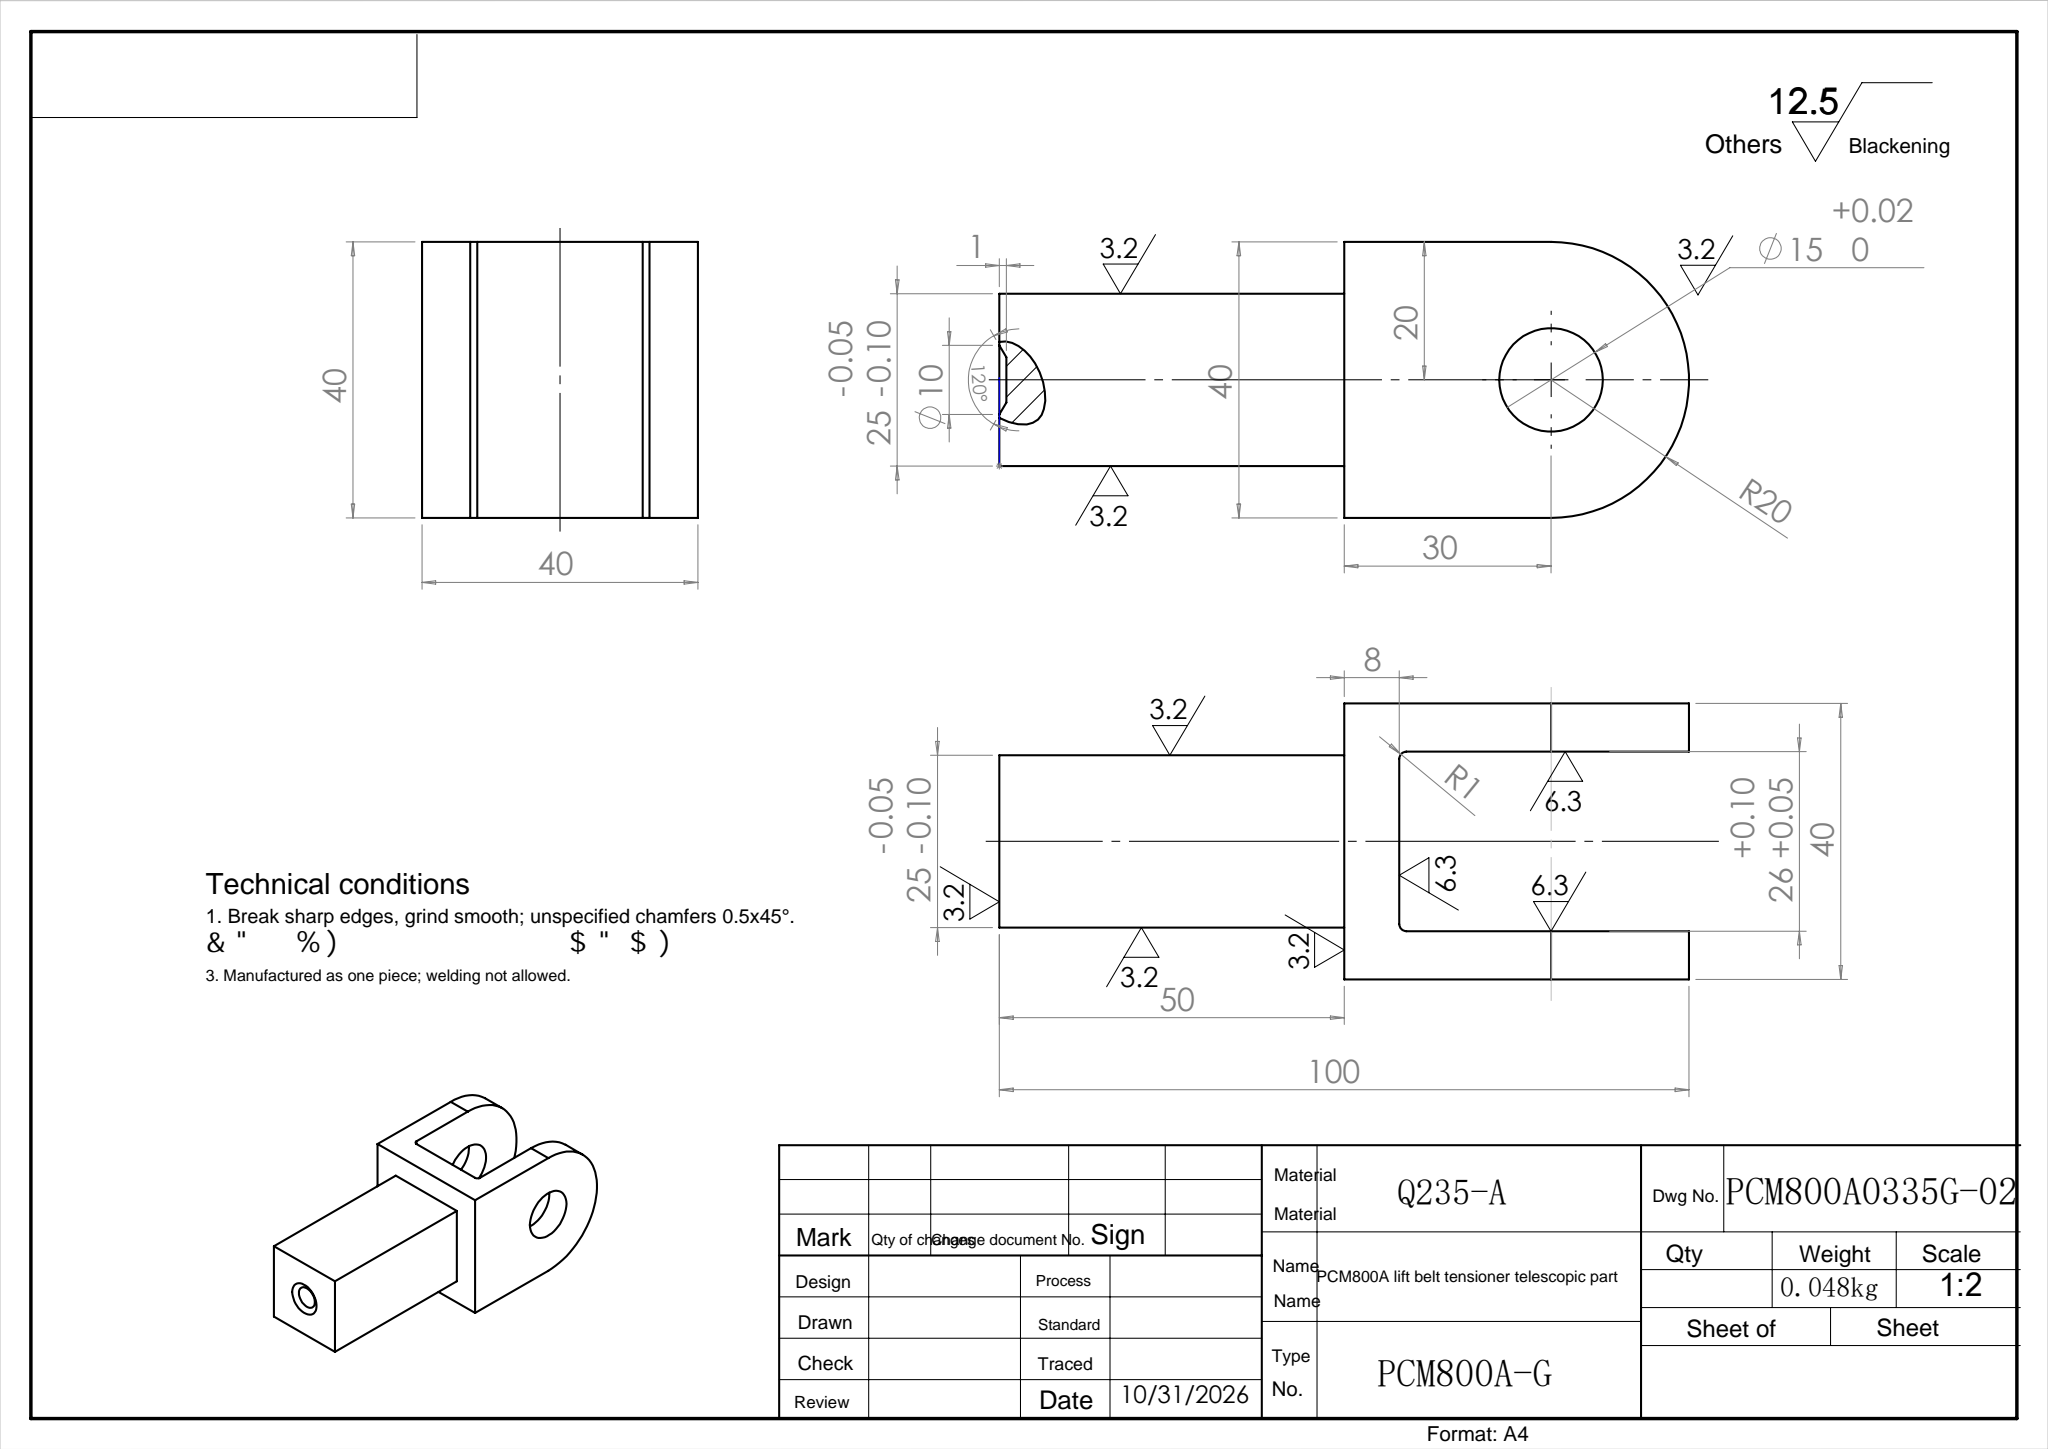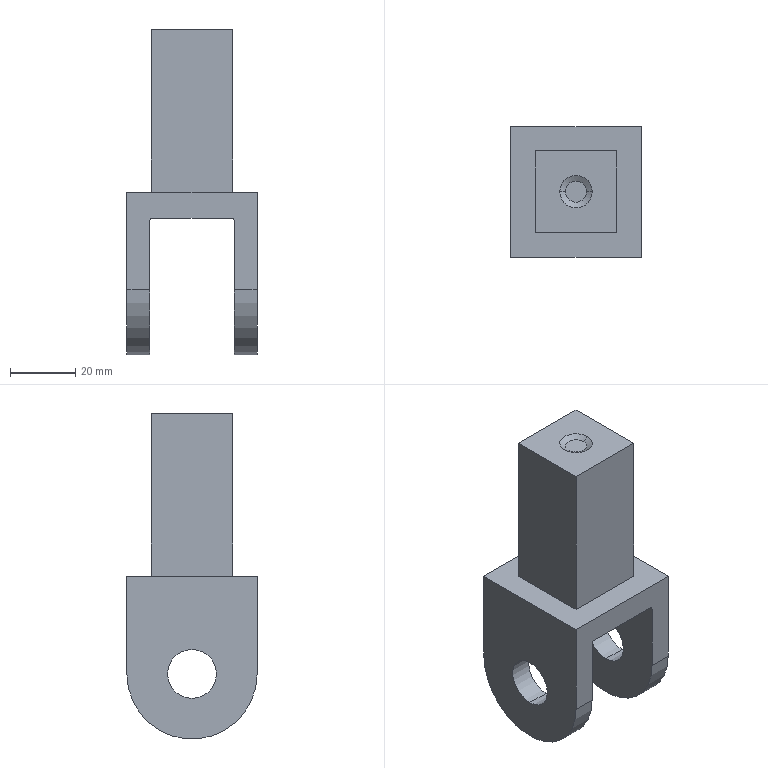Part | SolidWorks | features Fillet 1, MirrorStock 1 | 1 solid | 24 faces | box 40 x 40 x 100 mm | volume 62655 mm3 | plane 14 | cylinder 8 | cone 2 | commonest cylinder face diameters 15 x4 2 x2 40 x2
STEP:
#1=CARTESIAN_POINT('',(9.232,12.5,-1.));
#2=VERTEX_POINT('',#1);
#3=CARTESIAN_POINT('',(15.768,12.5,-1.));
#4=VERTEX_POINT('',#3);
#5=CARTESIAN_POINT('',(12.5,12.5,-1.));
#6=DIRECTION('',(0.,0.,-1.));
#7=DIRECTION('',(-1.,0.,0.));
#8=AXIS2_PLACEMENT_3D('',#5,#6,#7);
#9=CIRCLE('',#8,3.268);
#10=EDGE_CURVE('',#2,#4,#9,.T.);
#11=ORIENTED_EDGE('',*,*,#10,.T.);
#12=CARTESIAN_POINT('',(17.5,12.5,0.));
#13=VERTEX_POINT('',#12);
#14=CARTESIAN_POINT('',(17.5,12.5,0.));
#15=DIRECTION('',(0.866,0.,0.5));
#16=VECTOR('',#15,1000.);
#17=LINE('',#14,#16);
#18=EDGE_CURVE('',#4,#13,#17,.T.);
#19=ORIENTED_EDGE('',*,*,#18,.T.);
#20=CARTESIAN_POINT('',(7.5,12.5,0.));
#21=VERTEX_POINT('',#20);
#22=CARTESIAN_POINT('',(12.5,12.5,0.));
#23=DIRECTION('',(0.,0.,-1.));
#24=DIRECTION('',(-1.,0.,0.));
#25=AXIS2_PLACEMENT_3D('',#22,#23,#24);
#26=CIRCLE('',#25,5.);
#27=EDGE_CURVE('',#21,#13,#26,.T.);
#28=ORIENTED_EDGE('',*,*,#27,.F.);
#29=CARTESIAN_POINT('',(7.5,12.5,0.));
#30=DIRECTION('',(-0.866,0.,0.5));
#31=VECTOR('',#30,1000.);
#32=LINE('',#29,#31);
#33=EDGE_CURVE('',#2,#21,#32,.T.);
#34=ORIENTED_EDGE('',*,*,#33,.F.);
#35=EDGE_LOOP('',(#11,#19,#28,#34));
#36=FACE_OUTER_BOUND('',#35,.T.);
#37=CARTESIAN_POINT('',(12.5,12.5,0.));
#38=DIRECTION('',(0.,0.,1.));
#39=DIRECTION('',(-1.,0.,0.));
#40=AXIS2_PLACEMENT_3D('',#37,#38,#39);
#41=CONICAL_SURFACE('',#40,5.,1.047);
#42=ADVANCED_FACE('',(#36),#41,.F.);
#43=CARTESIAN_POINT('',(25.5,12.5,-72.5));
#44=VERTEX_POINT('',#43);
#45=CARTESIAN_POINT('',(25.5,12.5,-87.5));
#46=VERTEX_POINT('',#45);
#47=CARTESIAN_POINT('',(25.5,12.5,-80.));
#48=DIRECTION('',(-1.,0.,0.));
#49=DIRECTION('',(0.,1.,0.));
#50=AXIS2_PLACEMENT_3D('',#47,#48,#49);
#51=CIRCLE('',#50,7.5);
#52=EDGE_CURVE('',#44,#46,#51,.T.);
#53=ORIENTED_EDGE('',*,*,#52,.T.);
#54=CARTESIAN_POINT('',(32.5,12.5,-87.5));
#55=VERTEX_POINT('',#54);
#56=CARTESIAN_POINT('',(-7.5,12.5,-87.5));
#57=DIRECTION('',(1.,0.,0.));
#58=VECTOR('',#57,1000.);
#59=LINE('',#56,#58);
#60=EDGE_CURVE('',#46,#55,#59,.T.);
#61=ORIENTED_EDGE('',*,*,#60,.T.);
#62=CARTESIAN_POINT('',(32.5,12.5,-72.5));
#63=VERTEX_POINT('',#62);
#64=CARTESIAN_POINT('',(32.5,12.5,-80.));
#65=DIRECTION('',(-1.,0.,0.));
#66=DIRECTION('',(0.,0.,1.));
#67=AXIS2_PLACEMENT_3D('',#64,#65,#66);
#68=CIRCLE('',#67,7.5);
#69=EDGE_CURVE('',#63,#55,#68,.T.);
#70=ORIENTED_EDGE('',*,*,#69,.F.);
#71=CARTESIAN_POINT('',(-7.5,12.5,-72.5));
#72=DIRECTION('',(1.,0.,0.));
#73=VECTOR('',#72,1000.);
#74=LINE('',#71,#73);
#75=EDGE_CURVE('',#44,#63,#74,.T.);
#76=ORIENTED_EDGE('',*,*,#75,.F.);
#77=EDGE_LOOP('',(#53,#61,#70,#76));
#78=FACE_OUTER_BOUND('',#77,.T.);
#79=CARTESIAN_POINT('',(-7.5,12.5,-80.));
#80=DIRECTION('',(1.,0.,0.));
#81=DIRECTION('',(0.,0.,1.));
#82=AXIS2_PLACEMENT_3D('',#79,#80,#81);
#83=CYLINDRICAL_SURFACE('',#82,7.5);
#84=ADVANCED_FACE('',(#78),#83,.F.);
#85=CARTESIAN_POINT('',(-7.5,12.5,-72.5));
#86=VERTEX_POINT('',#85);
#87=CARTESIAN_POINT('',(-7.5,12.5,-87.5));
#88=VERTEX_POINT('',#87);
#89=CARTESIAN_POINT('',(-7.5,12.5,-80.));
#90=DIRECTION('',(-1.,0.,0.));
#91=DIRECTION('',(0.,0.,1.));
#92=AXIS2_PLACEMENT_3D('',#89,#90,#91);
#93=CIRCLE('',#92,7.5);
#94=EDGE_CURVE('',#86,#88,#93,.T.);
#95=ORIENTED_EDGE('',*,*,#94,.T.);
#96=CARTESIAN_POINT('',(-0.5,12.5,-87.5));
#97=VERTEX_POINT('',#96);
#98=CARTESIAN_POINT('',(-7.5,12.5,-87.5));
#99=DIRECTION('',(1.,0.,0.));
#100=VECTOR('',#99,1000.);
#101=LINE('',#98,#100);
#102=EDGE_CURVE('',#88,#97,#101,.T.);
#103=ORIENTED_EDGE('',*,*,#102,.T.);
#104=CARTESIAN_POINT('',(-0.5,12.5,-72.5));
#105=VERTEX_POINT('',#104);
#106=CARTESIAN_POINT('',(-0.5,12.5,-80.));
#107=DIRECTION('',(1.,0.,0.));
#108=DIRECTION('',(0.,-1.,0.));
#109=AXIS2_PLACEMENT_3D('',#106,#107,#108);
#110=CIRCLE('',#109,7.5);
#111=EDGE_CURVE('',#97,#105,#110,.T.);
#112=ORIENTED_EDGE('',*,*,#111,.T.);
#113=CARTESIAN_POINT('',(-7.5,12.5,-72.5));
#114=DIRECTION('',(1.,0.,0.));
#115=VECTOR('',#114,1000.);
#116=LINE('',#113,#115);
#117=EDGE_CURVE('',#86,#105,#116,.T.);
#118=ORIENTED_EDGE('',*,*,#117,.F.);
#119=EDGE_LOOP('',(#95,#103,#112,#118));
#120=FACE_OUTER_BOUND('',#119,.T.);
#121=CARTESIAN_POINT('',(-7.5,12.5,-80.));
#122=DIRECTION('',(1.,0.,0.));
#123=DIRECTION('',(0.,0.,1.));
#124=AXIS2_PLACEMENT_3D('',#121,#122,#123);
#125=CYLINDRICAL_SURFACE('',#124,7.5);
#126=ADVANCED_FACE('',(#120),#125,.F.);
#127=CARTESIAN_POINT('',(25.5,-7.5,-80.));
#128=VERTEX_POINT('',#127);
#129=CARTESIAN_POINT('',(25.5,32.5,-80.));
#130=VERTEX_POINT('',#129);
#131=CARTESIAN_POINT('',(25.5,12.5,-80.));
#132=DIRECTION('',(1.,0.,0.));
#133=DIRECTION('',(0.,1.,0.));
#134=AXIS2_PLACEMENT_3D('',#131,#132,#133);
#135=CIRCLE('',#134,20.);
#136=EDGE_CURVE('',#128,#130,#135,.T.);
#137=ORIENTED_EDGE('',*,*,#136,.T.);
#138=CARTESIAN_POINT('',(32.5,32.5,-80.));
#139=VERTEX_POINT('',#138);
#140=CARTESIAN_POINT('',(-17.5,32.5,-80.));
#141=DIRECTION('',(1.,0.,0.));
#142=VECTOR('',#141,1000.);
#143=LINE('',#140,#142);
#144=EDGE_CURVE('',#130,#139,#143,.T.);
#145=ORIENTED_EDGE('',*,*,#144,.T.);
#146=CARTESIAN_POINT('',(32.5,-7.5,-80.));
#147=VERTEX_POINT('',#146);
#148=CARTESIAN_POINT('',(32.5,12.5,-80.));
#149=DIRECTION('',(-1.,0.,0.));
#150=DIRECTION('',(0.,0.,1.));
#151=AXIS2_PLACEMENT_3D('',#148,#149,#150);
#152=CIRCLE('',#151,20.);
#153=EDGE_CURVE('',#139,#147,#152,.T.);
#154=ORIENTED_EDGE('',*,*,#153,.T.);
#155=CARTESIAN_POINT('',(-17.5,-7.5,-80.));
#156=DIRECTION('',(1.,0.,0.));
#157=VECTOR('',#156,1000.);
#158=LINE('',#155,#157);
#159=EDGE_CURVE('',#128,#147,#158,.T.);
#160=ORIENTED_EDGE('',*,*,#159,.F.);
#161=EDGE_LOOP('',(#137,#145,#154,#160));
#162=FACE_OUTER_BOUND('',#161,.T.);
#163=CARTESIAN_POINT('',(-17.5,12.5,-80.));
#164=DIRECTION('',(1.,0.,0.));
#165=DIRECTION('',(0.,0.,1.));
#166=AXIS2_PLACEMENT_3D('',#163,#164,#165);
#167=CYLINDRICAL_SURFACE('',#166,20.);
#168=ADVANCED_FACE('',(#162),#167,.T.);
#169=ORIENTED_EDGE('',*,*,#94,.F.);
#170=CARTESIAN_POINT('',(-7.5,12.5,-80.));
#171=DIRECTION('',(-1.,0.,0.));
#172=DIRECTION('',(0.,0.,1.));
#173=AXIS2_PLACEMENT_3D('',#170,#171,#172);
#174=CIRCLE('',#173,7.5);
#175=EDGE_CURVE('',#88,#86,#174,.T.);
#176=ORIENTED_EDGE('',*,*,#175,.F.);
#177=EDGE_LOOP('',(#169,#176));
#178=FACE_BOUND('',#177,.T.);
#179=CARTESIAN_POINT('',(-7.5,32.5,-80.));
#180=VERTEX_POINT('',#179);
#181=CARTESIAN_POINT('',(-7.5,-7.5,-80.));
#182=VERTEX_POINT('',#181);
#183=CARTESIAN_POINT('',(-7.5,12.5,-80.));
#184=DIRECTION('',(-1.,0.,0.));
#185=DIRECTION('',(0.,1.,0.));
#186=AXIS2_PLACEMENT_3D('',#183,#184,#185);
#187=CIRCLE('',#186,20.);
#188=EDGE_CURVE('',#180,#182,#187,.T.);
#189=ORIENTED_EDGE('',*,*,#188,.T.);
#190=CARTESIAN_POINT('',(-7.5,-7.5,-50.));
#191=VERTEX_POINT('',#190);
#192=CARTESIAN_POINT('',(-7.5,-7.5,-100.));
#193=DIRECTION('',(0.,0.,1.));
#194=VECTOR('',#193,1000.);
#195=LINE('',#192,#194);
#196=EDGE_CURVE('',#182,#191,#195,.T.);
#197=ORIENTED_EDGE('',*,*,#196,.T.);
#198=CARTESIAN_POINT('',(-7.5,32.5,-50.));
#199=VERTEX_POINT('',#198);
#200=CARTESIAN_POINT('',(-7.5,32.5,-50.));
#201=DIRECTION('',(0.,-1.,0.));
#202=VECTOR('',#201,1000.);
#203=LINE('',#200,#202);
#204=EDGE_CURVE('',#199,#191,#203,.T.);
#205=ORIENTED_EDGE('',*,*,#204,.F.);
#206=CARTESIAN_POINT('',(-7.5,32.5,-100.));
#207=DIRECTION('',(0.,0.,1.));
#208=VECTOR('',#207,1000.);
#209=LINE('',#206,#208);
#210=EDGE_CURVE('',#180,#199,#209,.T.);
#211=ORIENTED_EDGE('',*,*,#210,.F.);
#212=EDGE_LOOP('',(#189,#197,#205,#211));
#213=FACE_OUTER_BOUND('',#212,.T.);
#214=CARTESIAN_POINT('',(-7.5,32.5,-100.));
#215=DIRECTION('',(1.,0.,0.));
#216=DIRECTION('',(0.,1.,0.));
#217=AXIS2_PLACEMENT_3D('',#214,#215,#216);
#218=PLANE('',#217);
#219=ADVANCED_FACE('',(#178,#213),#218,.F.);
#220=ORIENTED_EDGE('',*,*,#69,.T.);
#221=CARTESIAN_POINT('',(32.5,12.5,-80.));
#222=DIRECTION('',(-1.,0.,0.));
#223=DIRECTION('',(0.,0.,1.));
#224=AXIS2_PLACEMENT_3D('',#221,#222,#223);
#225=CIRCLE('',#224,7.5);
#226=EDGE_CURVE('',#55,#63,#225,.T.);
#227=ORIENTED_EDGE('',*,*,#226,.T.);
#228=EDGE_LOOP('',(#220,#227));
#229=FACE_BOUND('',#228,.T.);
#230=CARTESIAN_POINT('',(32.5,32.5,-50.));
#231=VERTEX_POINT('',#230);
#232=CARTESIAN_POINT('',(32.5,32.5,-100.));
#233=DIRECTION('',(0.,0.,1.));
#234=VECTOR('',#233,1000.);
#235=LINE('',#232,#234);
#236=EDGE_CURVE('',#139,#231,#235,.T.);
#237=ORIENTED_EDGE('',*,*,#236,.T.);
#238=CARTESIAN_POINT('',(32.5,-7.5,-50.));
#239=VERTEX_POINT('',#238);
#240=CARTESIAN_POINT('',(32.5,32.5,-50.));
#241=DIRECTION('',(0.,1.,0.));
#242=VECTOR('',#241,1000.);
#243=LINE('',#240,#242);
#244=EDGE_CURVE('',#239,#231,#243,.T.);
#245=ORIENTED_EDGE('',*,*,#244,.F.);
#246=CARTESIAN_POINT('',(32.5,-7.5,-100.));
#247=DIRECTION('',(0.,0.,1.));
#248=VECTOR('',#247,1000.);
#249=LINE('',#246,#248);
#250=EDGE_CURVE('',#147,#239,#249,.T.);
#251=ORIENTED_EDGE('',*,*,#250,.F.);
#252=ORIENTED_EDGE('',*,*,#153,.F.);
#253=EDGE_LOOP('',(#237,#245,#251,#252));
#254=FACE_OUTER_BOUND('',#253,.T.);
#255=CARTESIAN_POINT('',(32.5,32.5,-100.));
#256=DIRECTION('',(-1.,0.,0.));
#257=DIRECTION('',(0.,0.,-1.));
#258=AXIS2_PLACEMENT_3D('',#255,#256,#257);
#259=PLANE('',#258);
#260=ADVANCED_FACE('',(#229,#254),#259,.F.);
#261=ORIENTED_EDGE('',*,*,#159,.T.);
#262=ORIENTED_EDGE('',*,*,#250,.T.);
#263=CARTESIAN_POINT('',(-7.5,-7.5,-50.));
#264=DIRECTION('',(1.,0.,0.));
#265=VECTOR('',#264,1000.);
#266=LINE('',#263,#265);
#267=EDGE_CURVE('',#191,#239,#266,.T.);
#268=ORIENTED_EDGE('',*,*,#267,.F.);
#269=ORIENTED_EDGE('',*,*,#196,.F.);
#270=CARTESIAN_POINT('',(-0.5,-7.5,-80.));
#271=VERTEX_POINT('',#270);
#272=CARTESIAN_POINT('',(-17.5,-7.5,-80.));
#273=DIRECTION('',(1.,0.,0.));
#274=VECTOR('',#273,1000.);
#275=LINE('',#272,#274);
#276=EDGE_CURVE('',#182,#271,#275,.T.);
#277=ORIENTED_EDGE('',*,*,#276,.T.);
#278=CARTESIAN_POINT('',(-0.5,-7.5,-59.));
#279=VERTEX_POINT('',#278);
#280=CARTESIAN_POINT('',(-0.5,-7.5,-58.));
#281=DIRECTION('',(0.,0.,-1.));
#282=VECTOR('',#281,1000.);
#283=LINE('',#280,#282);
#284=EDGE_CURVE('',#279,#271,#283,.T.);
#285=ORIENTED_EDGE('',*,*,#284,.F.);
#286=CARTESIAN_POINT('',(0.5,-7.5,-58.));
#287=VERTEX_POINT('',#286);
#288=CARTESIAN_POINT('',(0.5,-7.5,-59.));
#289=DIRECTION('',(0.,1.,0.));
#290=DIRECTION('',(0.,0.,1.));
#291=AXIS2_PLACEMENT_3D('',#288,#289,#290);
#292=CIRCLE('',#291,1.);
#293=EDGE_CURVE('',#279,#287,#292,.T.);
#294=ORIENTED_EDGE('',*,*,#293,.T.);
#295=CARTESIAN_POINT('',(24.5,-7.5,-58.));
#296=VERTEX_POINT('',#295);
#297=CARTESIAN_POINT('',(25.5,-7.5,-58.));
#298=DIRECTION('',(-1.,0.,0.));
#299=VECTOR('',#298,1000.);
#300=LINE('',#297,#299);
#301=EDGE_CURVE('',#296,#287,#300,.T.);
#302=ORIENTED_EDGE('',*,*,#301,.F.);
#303=CARTESIAN_POINT('',(25.5,-7.5,-59.));
#304=VERTEX_POINT('',#303);
#305=CARTESIAN_POINT('',(24.5,-7.5,-59.));
#306=DIRECTION('',(0.,1.,0.));
#307=DIRECTION('',(0.,0.,1.));
#308=AXIS2_PLACEMENT_3D('',#305,#306,#307);
#309=CIRCLE('',#308,1.);
#310=EDGE_CURVE('',#296,#304,#309,.T.);
#311=ORIENTED_EDGE('',*,*,#310,.T.);
#312=CARTESIAN_POINT('',(25.5,-7.5,-58.));
#313=DIRECTION('',(0.,0.,1.));
#314=VECTOR('',#313,1000.);
#315=LINE('',#312,#314);
#316=EDGE_CURVE('',#128,#304,#315,.T.);
#317=ORIENTED_EDGE('',*,*,#316,.F.);
#318=EDGE_LOOP('',(#261,#262,#268,#269,#277,#285,#294,#302,#311,#317));
#319=FACE_OUTER_BOUND('',#318,.T.);
#320=CARTESIAN_POINT('',(-7.5,-7.5,-100.));
#321=DIRECTION('',(0.,1.,0.));
#322=DIRECTION('',(0.,0.,-1.));
#323=AXIS2_PLACEMENT_3D('',#320,#321,#322);
#324=PLANE('',#323);
#325=ADVANCED_FACE('',(#319),#324,.F.);
#326=CARTESIAN_POINT('',(0.,25.,0.));
#327=VERTEX_POINT('',#326);
#328=CARTESIAN_POINT('',(0.,0.,0.));
#329=VERTEX_POINT('',#328);
#330=CARTESIAN_POINT('',(0.,0.,0.));
#331=DIRECTION('',(0.,-1.,0.));
#332=VECTOR('',#331,1000.);
#333=LINE('',#330,#332);
#334=EDGE_CURVE('',#327,#329,#333,.T.);
#335=ORIENTED_EDGE('',*,*,#334,.F.);
#336=CARTESIAN_POINT('',(0.,25.,-50.));
#337=VERTEX_POINT('',#336);
#338=CARTESIAN_POINT('',(0.,25.,-50.));
#339=DIRECTION('',(0.,0.,1.));
#340=VECTOR('',#339,1000.);
#341=LINE('',#338,#340);
#342=EDGE_CURVE('',#337,#327,#341,.T.);
#343=ORIENTED_EDGE('',*,*,#342,.F.);
#344=CARTESIAN_POINT('',(0.,0.,-50.));
#345=VERTEX_POINT('',#344);
#346=CARTESIAN_POINT('',(0.,0.,-50.));
#347=DIRECTION('',(0.,-1.,0.));
#348=VECTOR('',#347,1000.);
#349=LINE('',#346,#348);
#350=EDGE_CURVE('',#337,#345,#349,.T.);
#351=ORIENTED_EDGE('',*,*,#350,.T.);
#352=CARTESIAN_POINT('',(0.,0.,-50.));
#353=DIRECTION('',(0.,0.,1.));
#354=VECTOR('',#353,1000.);
#355=LINE('',#352,#354);
#356=EDGE_CURVE('',#345,#329,#355,.T.);
#357=ORIENTED_EDGE('',*,*,#356,.T.);
#358=EDGE_LOOP('',(#335,#343,#351,#357));
#359=FACE_OUTER_BOUND('',#358,.T.);
#360=CARTESIAN_POINT('',(0.,0.,-50.));
#361=DIRECTION('',(1.,0.,0.));
#362=DIRECTION('',(0.,0.,1.));
#363=AXIS2_PLACEMENT_3D('',#360,#361,#362);
#364=PLANE('',#363);
#365=ADVANCED_FACE('',(#359),#364,.F.);
#366=CARTESIAN_POINT('',(25.,0.,0.));
#367=VERTEX_POINT('',#366);
#368=CARTESIAN_POINT('',(0.,0.,0.));
#369=DIRECTION('',(1.,0.,0.));
#370=VECTOR('',#369,1000.);
#371=LINE('',#368,#370);
#372=EDGE_CURVE('',#329,#367,#371,.T.);
#373=ORIENTED_EDGE('',*,*,#372,.F.);
#374=ORIENTED_EDGE('',*,*,#356,.F.);
#375=CARTESIAN_POINT('',(25.,0.,-50.));
#376=VERTEX_POINT('',#375);
#377=CARTESIAN_POINT('',(0.,0.,-50.));
#378=DIRECTION('',(1.,0.,0.));
#379=VECTOR('',#378,1000.);
#380=LINE('',#377,#379);
#381=EDGE_CURVE('',#345,#376,#380,.T.);
#382=ORIENTED_EDGE('',*,*,#381,.T.);
#383=CARTESIAN_POINT('',(25.,0.,-50.));
#384=DIRECTION('',(0.,0.,1.));
#385=VECTOR('',#384,1000.);
#386=LINE('',#383,#385);
#387=EDGE_CURVE('',#376,#367,#386,.T.);
#388=ORIENTED_EDGE('',*,*,#387,.T.);
#389=EDGE_LOOP('',(#373,#374,#382,#388));
#390=FACE_OUTER_BOUND('',#389,.T.);
#391=CARTESIAN_POINT('',(0.,0.,-50.));
#392=DIRECTION('',(0.,1.,0.));
#393=DIRECTION('',(0.,0.,-1.));
#394=AXIS2_PLACEMENT_3D('',#391,#392,#393);
#395=PLANE('',#394);
#396=ADVANCED_FACE('',(#390),#395,.F.);
#397=CARTESIAN_POINT('',(25.,25.,0.));
#398=VERTEX_POINT('',#397);
#399=CARTESIAN_POINT('',(25.,0.,0.));
#400=DIRECTION('',(0.,1.,0.));
#401=VECTOR('',#400,1000.);
#402=LINE('',#399,#401);
#403=EDGE_CURVE('',#367,#398,#402,.T.);
#404=ORIENTED_EDGE('',*,*,#403,.F.);
#405=ORIENTED_EDGE('',*,*,#387,.F.);
#406=CARTESIAN_POINT('',(25.,25.,-50.));
#407=VERTEX_POINT('',#406);
#408=CARTESIAN_POINT('',(25.,0.,-50.));
#409=DIRECTION('',(0.,1.,0.));
#410=VECTOR('',#409,1000.);
#411=LINE('',#408,#410);
#412=EDGE_CURVE('',#376,#407,#411,.T.);
#413=ORIENTED_EDGE('',*,*,#412,.T.);
#414=CARTESIAN_POINT('',(25.,25.,-50.));
#415=DIRECTION('',(0.,0.,1.));
#416=VECTOR('',#415,1000.);
#417=LINE('',#414,#416);
#418=EDGE_CURVE('',#407,#398,#417,.T.);
#419=ORIENTED_EDGE('',*,*,#418,.T.);
#420=EDGE_LOOP('',(#404,#405,#413,#419));
#421=FACE_OUTER_BOUND('',#420,.T.);
#422=CARTESIAN_POINT('',(25.,0.,-50.));
#423=DIRECTION('',(-1.,0.,0.));
#424=DIRECTION('',(0.,0.,-1.));
#425=AXIS2_PLACEMENT_3D('',#422,#423,#424);
#426=PLANE('',#425);
#427=ADVANCED_FACE('',(#421),#426,.F.);
#428=CARTESIAN_POINT('',(0.,25.,0.));
#429=DIRECTION('',(-1.,0.,0.));
#430=VECTOR('',#429,1000.);
#431=LINE('',#428,#430);
#432=EDGE_CURVE('',#398,#327,#431,.T.);
#433=ORIENTED_EDGE('',*,*,#432,.F.);
#434=ORIENTED_EDGE('',*,*,#418,.F.);
#435=CARTESIAN_POINT('',(0.,25.,-50.));
#436=DIRECTION('',(-1.,0.,0.));
#437=VECTOR('',#436,1000.);
#438=LINE('',#435,#437);
#439=EDGE_CURVE('',#407,#337,#438,.T.);
#440=ORIENTED_EDGE('',*,*,#439,.T.);
#441=ORIENTED_EDGE('',*,*,#342,.T.);
#442=EDGE_LOOP('',(#433,#434,#440,#441));
#443=FACE_OUTER_BOUND('',#442,.T.);
#444=CARTESIAN_POINT('',(0.,25.,-50.));
#445=DIRECTION('',(0.,-1.,0.));
#446=DIRECTION('',(0.,0.,1.));
#447=AXIS2_PLACEMENT_3D('',#444,#445,#446);
#448=PLANE('',#447);
#449=ADVANCED_FACE('',(#443),#448,.F.);
#450=ORIENTED_EDGE('',*,*,#27,.T.);
#451=CARTESIAN_POINT('',(12.5,12.5,0.));
#452=DIRECTION('',(0.,0.,-1.));
#453=DIRECTION('',(-1.,0.,0.));
#454=AXIS2_PLACEMENT_3D('',#451,#452,#453);
#455=CIRCLE('',#454,5.);
#456=EDGE_CURVE('',#13,#21,#455,.T.);
#457=ORIENTED_EDGE('',*,*,#456,.T.);
#458=EDGE_LOOP('',(#450,#457));
#459=FACE_BOUND('',#458,.T.);
#460=ORIENTED_EDGE('',*,*,#334,.T.);
#461=ORIENTED_EDGE('',*,*,#372,.T.);
#462=ORIENTED_EDGE('',*,*,#403,.T.);
#463=ORIENTED_EDGE('',*,*,#432,.T.);
#464=EDGE_LOOP('',(#460,#461,#462,#463));
#465=FACE_OUTER_BOUND('',#464,.T.);
#466=CARTESIAN_POINT('',(0.,25.,0.));
#467=DIRECTION('',(0.,0.,1.));
#468=DIRECTION('',(-1.,0.,0.));
#469=AXIS2_PLACEMENT_3D('',#466,#467,#468);
#470=PLANE('',#469);
#471=ADVANCED_FACE('',(#459,#465),#470,.T.);
#472=ORIENTED_EDGE('',*,*,#204,.T.);
#473=ORIENTED_EDGE('',*,*,#267,.T.);
#474=ORIENTED_EDGE('',*,*,#244,.T.);
#475=CARTESIAN_POINT('',(-7.5,32.5,-50.));
#476=DIRECTION('',(-1.,0.,0.));
#477=VECTOR('',#476,1000.);
#478=LINE('',#475,#477);
#479=EDGE_CURVE('',#231,#199,#478,.T.);
#480=ORIENTED_EDGE('',*,*,#479,.T.);
#481=EDGE_LOOP('',(#472,#473,#474,#480));
#482=FACE_OUTER_BOUND('',#481,.T.);
#483=ORIENTED_EDGE('',*,*,#439,.F.);
#484=ORIENTED_EDGE('',*,*,#412,.F.);
#485=ORIENTED_EDGE('',*,*,#381,.F.);
#486=ORIENTED_EDGE('',*,*,#350,.F.);
#487=EDGE_LOOP('',(#483,#484,#485,#486));
#488=FACE_BOUND('',#487,.T.);
#489=CARTESIAN_POINT('',(-7.5,-7.5,-50.));
#490=DIRECTION('',(0.,0.,-1.));
#491=DIRECTION('',(1.,0.,0.));
#492=AXIS2_PLACEMENT_3D('',#489,#490,#491);
#493=PLANE('',#492);
#494=ADVANCED_FACE('',(#482,#488),#493,.F.);
#495=CARTESIAN_POINT('',(25.5,32.5,-59.));
#496=VERTEX_POINT('',#495);
#497=CARTESIAN_POINT('',(25.5,32.5,-58.));
#498=DIRECTION('',(0.,0.,1.));
#499=VECTOR('',#498,1000.);
#500=LINE('',#497,#499);
#501=EDGE_CURVE('',#130,#496,#500,.T.);
#502=ORIENTED_EDGE('',*,*,#501,.T.);
#503=CARTESIAN_POINT('',(24.5,32.5,-58.));
#504=VERTEX_POINT('',#503);
#505=CARTESIAN_POINT('',(24.5,32.5,-59.));
#506=DIRECTION('',(0.,-1.,0.));
#507=DIRECTION('',(1.,0.,0.));
#508=AXIS2_PLACEMENT_3D('',#505,#506,#507);
#509=CIRCLE('',#508,1.);
#510=EDGE_CURVE('',#496,#504,#509,.T.);
#511=ORIENTED_EDGE('',*,*,#510,.T.);
#512=CARTESIAN_POINT('',(0.5,32.5,-58.));
#513=VERTEX_POINT('',#512);
#514=CARTESIAN_POINT('',(25.5,32.5,-58.));
#515=DIRECTION('',(-1.,0.,0.));
#516=VECTOR('',#515,1000.);
#517=LINE('',#514,#516);
#518=EDGE_CURVE('',#504,#513,#517,.T.);
#519=ORIENTED_EDGE('',*,*,#518,.T.);
#520=CARTESIAN_POINT('',(-0.5,32.5,-59.));
#521=VERTEX_POINT('',#520);
#522=CARTESIAN_POINT('',(0.5,32.5,-59.));
#523=DIRECTION('',(0.,-1.,0.));
#524=DIRECTION('',(1.,0.,0.));
#525=AXIS2_PLACEMENT_3D('',#522,#523,#524);
#526=CIRCLE('',#525,1.);
#527=EDGE_CURVE('',#513,#521,#526,.T.);
#528=ORIENTED_EDGE('',*,*,#527,.T.);
#529=CARTESIAN_POINT('',(-0.5,32.5,-80.));
#530=VERTEX_POINT('',#529);
#531=CARTESIAN_POINT('',(-0.5,32.5,-58.));
#532=DIRECTION('',(0.,0.,-1.));
#533=VECTOR('',#532,1000.);
#534=LINE('',#531,#533);
#535=EDGE_CURVE('',#521,#530,#534,.T.);
#536=ORIENTED_EDGE('',*,*,#535,.T.);
#537=CARTESIAN_POINT('',(-17.5,32.5,-80.));
#538=DIRECTION('',(1.,0.,0.));
#539=VECTOR('',#538,1000.);
#540=LINE('',#537,#539);
#541=EDGE_CURVE('',#180,#530,#540,.T.);
#542=ORIENTED_EDGE('',*,*,#541,.F.);
#543=ORIENTED_EDGE('',*,*,#210,.T.);
#544=ORIENTED_EDGE('',*,*,#479,.F.);
#545=ORIENTED_EDGE('',*,*,#236,.F.);
#546=ORIENTED_EDGE('',*,*,#144,.F.);
#547=EDGE_LOOP('',(#502,#511,#519,#528,#536,#542,#543,#544,#545,#546));
#548=FACE_OUTER_BOUND('',#547,.T.);
#549=CARTESIAN_POINT('',(-7.5,32.5,-100.));
#550=DIRECTION('',(0.,-1.,0.));
#551=DIRECTION('',(1.,0.,0.));
#552=AXIS2_PLACEMENT_3D('',#549,#550,#551);
#553=PLANE('',#552);
#554=ADVANCED_FACE('',(#548),#553,.F.);
#555=CARTESIAN_POINT('',(-0.5,12.5,-80.));
#556=DIRECTION('',(-1.,0.,0.));
#557=DIRECTION('',(0.,-1.,0.));
#558=AXIS2_PLACEMENT_3D('',#555,#556,#557);
#559=CIRCLE('',#558,20.);
#560=EDGE_CURVE('',#530,#271,#559,.T.);
#561=ORIENTED_EDGE('',*,*,#560,.T.);
#562=ORIENTED_EDGE('',*,*,#276,.F.);
#563=ORIENTED_EDGE('',*,*,#188,.F.);
#564=ORIENTED_EDGE('',*,*,#541,.T.);
#565=EDGE_LOOP('',(#561,#562,#563,#564));
#566=FACE_OUTER_BOUND('',#565,.T.);
#567=CARTESIAN_POINT('',(-17.5,12.5,-80.));
#568=DIRECTION('',(1.,0.,0.));
#569=DIRECTION('',(0.,0.,1.));
#570=AXIS2_PLACEMENT_3D('',#567,#568,#569);
#571=CYLINDRICAL_SURFACE('',#570,20.);
#572=ADVANCED_FACE('',(#566),#571,.T.);
#573=ORIENTED_EDGE('',*,*,#52,.F.);
#574=CARTESIAN_POINT('',(25.5,12.5,-80.));
#575=DIRECTION('',(-1.,0.,0.));
#576=DIRECTION('',(0.,1.,0.));
#577=AXIS2_PLACEMENT_3D('',#574,#575,#576);
#578=CIRCLE('',#577,7.5);
#579=EDGE_CURVE('',#46,#44,#578,.T.);
#580=ORIENTED_EDGE('',*,*,#579,.F.);
#581=EDGE_LOOP('',(#573,#580));
#582=FACE_BOUND('',#581,.T.);
#583=ORIENTED_EDGE('',*,*,#316,.T.);
#584=CARTESIAN_POINT('',(25.5,32.5,-59.));
#585=DIRECTION('',(0.,1.,0.));
#586=VECTOR('',#585,1000.);
#587=LINE('',#584,#586);
#588=EDGE_CURVE('',#304,#496,#587,.T.);
#589=ORIENTED_EDGE('',*,*,#588,.T.);
#590=ORIENTED_EDGE('',*,*,#501,.F.);
#591=ORIENTED_EDGE('',*,*,#136,.F.);
#592=EDGE_LOOP('',(#583,#589,#590,#591));
#593=FACE_OUTER_BOUND('',#592,.T.);
#594=CARTESIAN_POINT('',(25.5,-7.5,-58.));
#595=DIRECTION('',(1.,0.,0.));
#596=DIRECTION('',(0.,1.,0.));
#597=AXIS2_PLACEMENT_3D('',#594,#595,#596);
#598=PLANE('',#597);
#599=ADVANCED_FACE('',(#582,#593),#598,.F.);
#600=CARTESIAN_POINT('',(-0.5,12.5,-80.));
#601=DIRECTION('',(1.,0.,0.));
#602=DIRECTION('',(0.,-1.,0.));
#603=AXIS2_PLACEMENT_3D('',#600,#601,#602);
#604=CIRCLE('',#603,7.5);
#605=EDGE_CURVE('',#105,#97,#604,.T.);
#606=ORIENTED_EDGE('',*,*,#605,.F.);
#607=ORIENTED_EDGE('',*,*,#111,.F.);
#608=EDGE_LOOP('',(#606,#607));
#609=FACE_BOUND('',#608,.T.);
#610=ORIENTED_EDGE('',*,*,#535,.F.);
#611=CARTESIAN_POINT('',(-0.5,-7.5,-59.));
#612=DIRECTION('',(0.,-1.,0.));
#613=VECTOR('',#612,1000.);
#614=LINE('',#611,#613);
#615=EDGE_CURVE('',#521,#279,#614,.T.);
#616=ORIENTED_EDGE('',*,*,#615,.T.);
#617=ORIENTED_EDGE('',*,*,#284,.T.);
#618=ORIENTED_EDGE('',*,*,#560,.F.);
#619=EDGE_LOOP('',(#610,#616,#617,#618));
#620=FACE_OUTER_BOUND('',#619,.T.);
#621=CARTESIAN_POINT('',(-0.5,-7.5,-58.));
#622=DIRECTION('',(-1.,0.,0.));
#623=DIRECTION('',(0.,-1.,0.));
#624=AXIS2_PLACEMENT_3D('',#621,#622,#623);
#625=PLANE('',#624);
#626=ADVANCED_FACE('',(#609,#620),#625,.F.);
#627=ORIENTED_EDGE('',*,*,#518,.F.);
#628=CARTESIAN_POINT('',(24.5,-7.5,-58.));
#629=DIRECTION('',(0.,-1.,0.));
#630=VECTOR('',#629,1000.);
#631=LINE('',#628,#630);
#632=EDGE_CURVE('',#504,#296,#631,.T.);
#633=ORIENTED_EDGE('',*,*,#632,.T.);
#634=ORIENTED_EDGE('',*,*,#301,.T.);
#635=CARTESIAN_POINT('',(0.5,32.5,-58.));
#636=DIRECTION('',(0.,1.,0.));
#637=VECTOR('',#636,1000.);
#638=LINE('',#635,#637);
#639=EDGE_CURVE('',#287,#513,#638,.T.);
#640=ORIENTED_EDGE('',*,*,#639,.T.);
#641=EDGE_LOOP('',(#627,#633,#634,#640));
#642=FACE_OUTER_BOUND('',#641,.T.);
#643=CARTESIAN_POINT('',(25.5,-7.5,-58.));
#644=DIRECTION('',(0.,0.,1.));
#645=DIRECTION('',(-1.,0.,0.));
#646=AXIS2_PLACEMENT_3D('',#643,#644,#645);
#647=PLANE('',#646);
#648=ADVANCED_FACE('',(#642),#647,.F.);
#649=ORIENTED_EDGE('',*,*,#102,.F.);
#650=ORIENTED_EDGE('',*,*,#175,.T.);
#651=ORIENTED_EDGE('',*,*,#117,.T.);
#652=ORIENTED_EDGE('',*,*,#605,.T.);
#653=EDGE_LOOP('',(#649,#650,#651,#652));
#654=FACE_OUTER_BOUND('',#653,.T.);
#655=CARTESIAN_POINT('',(-7.5,12.5,-80.));
#656=DIRECTION('',(1.,0.,0.));
#657=DIRECTION('',(0.,0.,1.));
#658=AXIS2_PLACEMENT_3D('',#655,#656,#657);
#659=CYLINDRICAL_SURFACE('',#658,7.5);
#660=ADVANCED_FACE('',(#654),#659,.F.);
#661=ORIENTED_EDGE('',*,*,#60,.F.);
#662=ORIENTED_EDGE('',*,*,#579,.T.);
#663=ORIENTED_EDGE('',*,*,#75,.T.);
#664=ORIENTED_EDGE('',*,*,#226,.F.);
#665=EDGE_LOOP('',(#661,#662,#663,#664));
#666=FACE_OUTER_BOUND('',#665,.T.);
#667=CARTESIAN_POINT('',(-7.5,12.5,-80.));
#668=DIRECTION('',(1.,0.,0.));
#669=DIRECTION('',(0.,0.,1.));
#670=AXIS2_PLACEMENT_3D('',#667,#668,#669);
#671=CYLINDRICAL_SURFACE('',#670,7.5);
#672=ADVANCED_FACE('',(#666),#671,.F.);
#673=ORIENTED_EDGE('',*,*,#18,.F.);
#674=CARTESIAN_POINT('',(12.5,12.5,-1.));
#675=DIRECTION('',(0.,0.,-1.));
#676=DIRECTION('',(-1.,0.,0.));
#677=AXIS2_PLACEMENT_3D('',#674,#675,#676);
#678=CIRCLE('',#677,3.268);
#679=EDGE_CURVE('',#4,#2,#678,.T.);
#680=ORIENTED_EDGE('',*,*,#679,.T.);
#681=ORIENTED_EDGE('',*,*,#33,.T.);
#682=ORIENTED_EDGE('',*,*,#456,.F.);
#683=EDGE_LOOP('',(#673,#680,#681,#682));
#684=FACE_OUTER_BOUND('',#683,.T.);
#685=CARTESIAN_POINT('',(12.5,12.5,0.));
#686=DIRECTION('',(0.,0.,1.));
#687=DIRECTION('',(-1.,0.,0.));
#688=AXIS2_PLACEMENT_3D('',#685,#686,#687);
#689=CONICAL_SURFACE('',#688,5.,1.047);
#690=ADVANCED_FACE('',(#684),#689,.F.);
#691=ORIENTED_EDGE('',*,*,#10,.F.);
#692=ORIENTED_EDGE('',*,*,#679,.F.);
#693=EDGE_LOOP('',(#691,#692));
#694=FACE_OUTER_BOUND('',#693,.T.);
#695=CARTESIAN_POINT('',(12.5,12.5,-1.));
#696=DIRECTION('',(0.,0.,1.));
#697=DIRECTION('',(-1.,0.,0.));
#698=AXIS2_PLACEMENT_3D('',#695,#696,#697);
#699=PLANE('',#698);
#700=ADVANCED_FACE('',(#694),#699,.T.);
#701=ORIENTED_EDGE('',*,*,#310,.F.);
#702=ORIENTED_EDGE('',*,*,#632,.F.);
#703=ORIENTED_EDGE('',*,*,#510,.F.);
#704=ORIENTED_EDGE('',*,*,#588,.F.);
#705=EDGE_LOOP('',(#701,#702,#703,#704));
#706=FACE_OUTER_BOUND('',#705,.T.);
#707=CARTESIAN_POINT('',(24.5,-7.5,-59.));
#708=DIRECTION('',(0.,-1.,0.));
#709=DIRECTION('',(1.,0.,0.));
#710=AXIS2_PLACEMENT_3D('',#707,#708,#709);
#711=CYLINDRICAL_SURFACE('',#710,1.);
#712=ADVANCED_FACE('',(#706),#711,.F.);
#713=ORIENTED_EDGE('',*,*,#293,.F.);
#714=ORIENTED_EDGE('',*,*,#615,.F.);
#715=ORIENTED_EDGE('',*,*,#527,.F.);
#716=ORIENTED_EDGE('',*,*,#639,.F.);
#717=EDGE_LOOP('',(#713,#714,#715,#716));
#718=FACE_OUTER_BOUND('',#717,.T.);
#719=CARTESIAN_POINT('',(0.5,-7.5,-59.));
#720=DIRECTION('',(0.,-1.,0.));
#721=DIRECTION('',(1.,0.,0.));
#722=AXIS2_PLACEMENT_3D('',#719,#720,#721);
#723=CYLINDRICAL_SURFACE('',#722,1.);
#724=ADVANCED_FACE('',(#718),#723,.F.);
#725=CLOSED_SHELL('',(#42,#84,#126,#168,#219,#260,#325,#365,#396,#427,#449,#471,#494,#554,#572,#599,#626,#648,#660,#672,#690,#700,#712,#724));
#726=MANIFOLD_SOLID_BREP('',#725);
#727=CARTESIAN_POINT('',(0.,0.,0.));
#728=DIRECTION('',(0.,0.,1.));
#729=DIRECTION('',(1.,0.,0.));
#730=AXIS2_PLACEMENT_3D('',#727,#728,#729);
#731=(LENGTH_UNIT()NAMED_UNIT(*)SI_UNIT(.MILLI.,.METRE.));
#732=UNCERTAINTY_MEASURE_WITH_UNIT(LENGTH_MEASURE(0.00001),#731,'','');
#733=(NAMED_UNIT(*)PLANE_ANGLE_UNIT()SI_UNIT($,.RADIAN.));
#734=(NAMED_UNIT(*)SI_UNIT($,.STERADIAN.)SOLID_ANGLE_UNIT());
#735=(GEOMETRIC_REPRESENTATION_CONTEXT(3)GLOBAL_UNCERTAINTY_ASSIGNED_CONTEXT((#732))GLOBAL_UNIT_ASSIGNED_CONTEXT((#731,#733,#734))REPRESENTATION_CONTEXT('',''));
#736=ADVANCED_BREP_SHAPE_REPRESENTATION('',(#726,#730),#735);